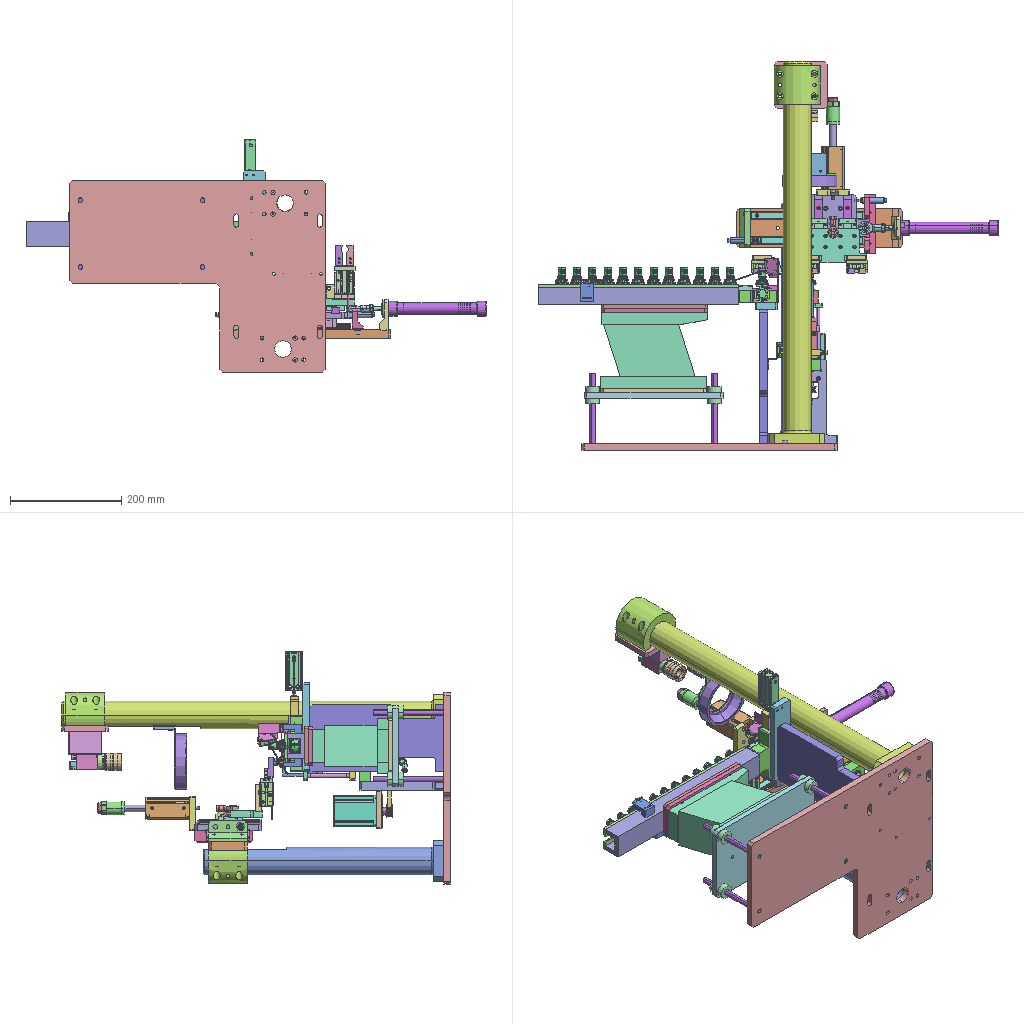Assembly | STEP file | 91 different items | 145 placed | box 828 x 700 x 418 mm
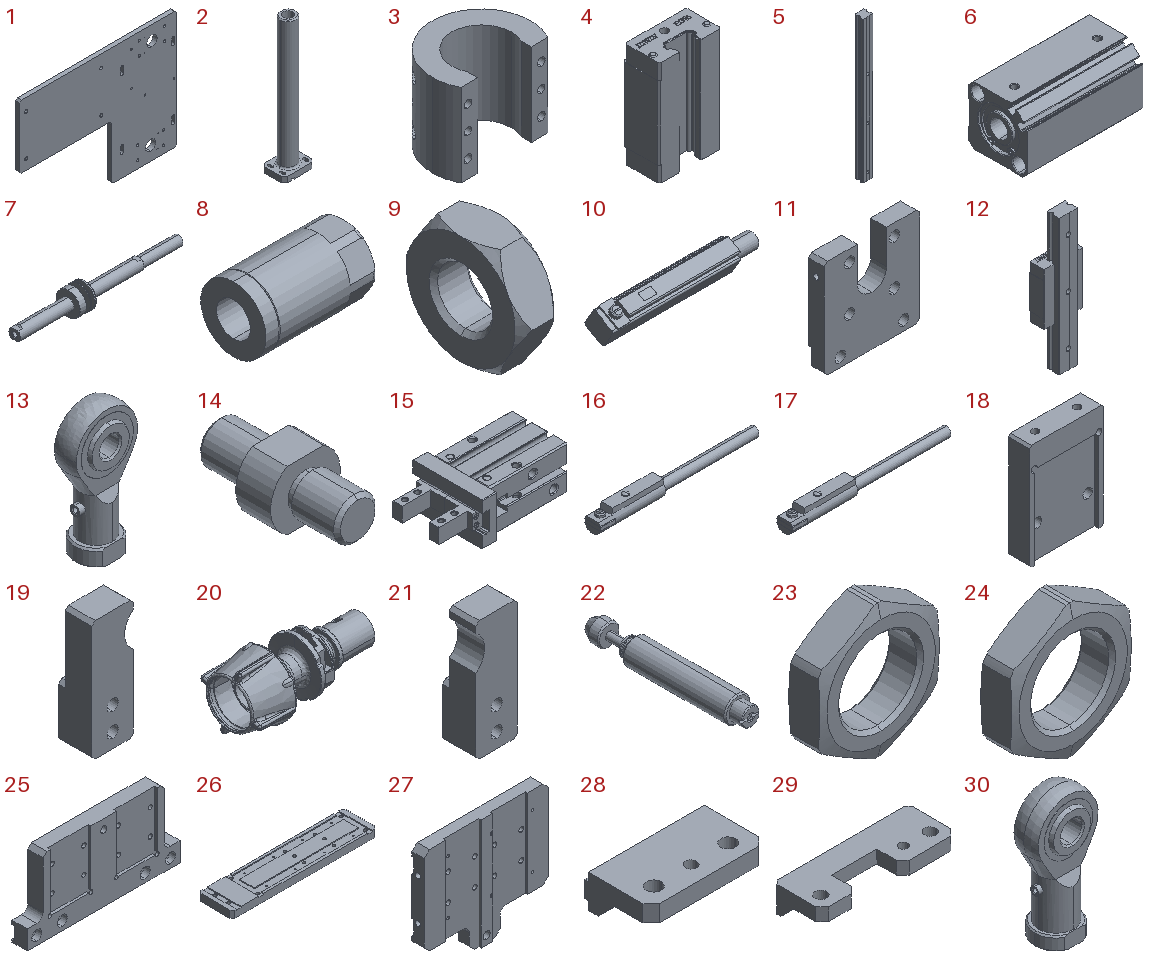Parts list (item | name | quantity | parent item | size | volume):
1 | PN_0009 | x1 | - | 460 x 12 x 345 mm | 1349018 mm3
2 | PN_0012 | x1 | in PN_0011 | 100 x 75 x 433 mm | 612416 mm3
3 | PN_0003 | x2 | in PN_0011, PN_0020 | 83 x 61 x 70 mm | 151269 mm3
4 | EGH15CA_BLOCK | x2 | in EGH15CA-220-2 | 34 x 19.5 x 57.8 mm | 30496 mm3
5 | EG15_RAIL-200 | x2 | in EGH15CA-220-2 | 15 x 12.5 x 200 mm | 32053 mm3
6 | ACQJS-25x40-20-G-11 | x1 | in ACQJS-25x40-20-G-1 (00) | 79 x 40 x 40 mm | 79327 mm3
7 | ACQJS-25x40-20-G-12 | x1 | in ACQJS-25x40-20-G-1 (00) | 170.5 x 25 x 25 mm | 21717 mm3
8 | ACQJS-25x40-20-G-13 | x1 | in ACQJS-25x40-20-G-1 (00) | 41 x 24 x 24 mm | 13745 mm3
9 | ACQJS-25x40-20-G-14 | x1 | in ACQJS-25x40-20-G-1 (00) | 6 x 19.63 x 17 mm | 1118 mm3
10 | ACQJS-25x40-20-G-15 | x1 | in ACQJS-25x40-20-G-1 (00) | 30.5 x 5.877 x 6.057 mm | 552.742 mm3
11 | PN_0013 | x1 | in PN_0011 | 60 x 10 x 62 mm | 28419 mm3
12 | MGN15C | x2 | in PN_0011 | 32 x 16 x 110 mm | 27183 mm3
13 | F-M06100U1 | x1 | in PN_0011 | - | 3624 mm3
14 | PN_0004 | x1 | in PN_0011 | 10 x 20 x 8.5 mm | 768.323 mm3
15 | HFZ16-B--BCL-H-21 | x3 | in HFZ16-B--BCL-H-2 | 67.3 x 38 x 23.6 mm | 30878 mm3
16 | HFZ16-B--BCL-H-22 | x3 | in HFZ16-B--BCL-H-2 | 42 x 4 x 5.1 mm | 360.74 mm3
17 | HFZ16-B--BCL-H-23 | x3 | in HFZ16-B--BCL-H-2 | 42 x 4 x 5.1 mm | 360.74 mm3
18 | PN_0014 | x3 | in PN_0011 | 35 x 10 x 50 mm | 14292 mm3
19 | PN_0015 | x3 | in PN_0011 | 12.5 x 10 x 36 mm | 3520 mm3
20 | Product 1 | x16 | in PN_0011, PN_0026, PN_0034, PN_0047 | 57.85 x 26.867 x 26.867 mm | 9145 mm3
21 | PN_0016 | x3 | in PN_0011 | 12.5 x 10 x 36 mm | 3520 mm3
22 | ACA-1007-11 | x2 | in ACA-1007-1 | 10 x 62 x 10 mm | 3798 mm3
23 | ACA-1007-12 | x2 | in ACA-1007-1 | 14 x 4 x 15.686 mm | 394.069 mm3
24 | ACA-1007-13 | x2 | in ACA-1007-1 | 14 x 4 x 15.686 mm | 394.069 mm3
25 | PN_0017 | x1 | in PN_0011 | 120 x 12 x 60 mm | 62781 mm3
26 | PN_0018 | x1 | in PN_0011 | 300 x 70 x 15 mm | 290778 mm3
27 | PN_0019 | x1 | in PN_0011 | 120 x 12 x 107.5 mm | 106389 mm3
28 | PN_0005 | x1 | in PN_0011 | 70 x 40 x 20 mm | 33206 mm3
29 | PN_0007 | x1 | in PN_0011 | 105 x 40 x 20 mm | 43466 mm3
30 | F-M08125U | x1 | in PN_0011 | 24 x 14 x 48 mm | 6722 mm3
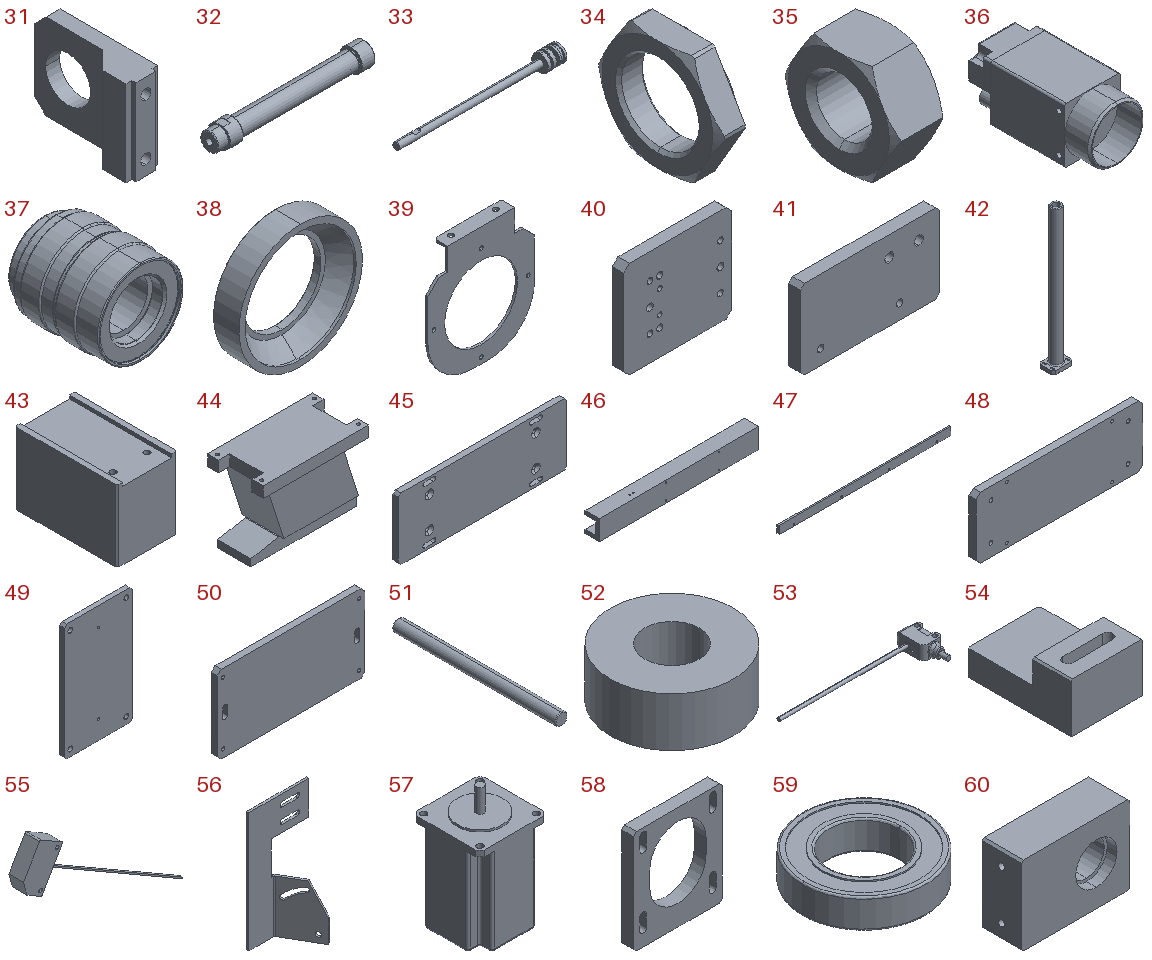31 | PN_0006 | x1 | in PN_0011 | 16 x 57 x 43 mm | 19963 mm3
32 | MA20x100-S-U1 | x1 | in MA20x100-S-U (0) | 188 x 27 x 27 mm | 33330 mm3
33 | MA20x100-S-U2 | x1 | in MA20x100-S-U (0) | 189 x 19.5 x 19.5 mm | 13401 mm3
34 | MA20x100-S-U3 | x1 | in MA20x100-S-U (0) | 7 x 33 x 29 mm | 2695 mm3
35 | MA20x100-S-U4 | x1 | in MA20x100-S-U (0) | 6 x 13.856 x 12 mm | 526.038 mm3
36 | MVC1000MF-M00 camera | x1 | in PN_0020 | 29 x 63.7 x 29 mm | 38507 mm3
37 | LTABA30_LTABA30 | x1 | in PN_0020 | 31 x 34 x 31 mm | 15140 mm3
38 | WLDR-LA100-W light source | x1 | in PN_0020 | 100 x 21 x 100 mm | 62526 mm3
39 | PN_0021 | x1 | in PN_0020 | 95 x 12 x 106 mm | 11586 mm3
40 | PN_0022 | x1 | in PN_0020 | 95 x 10 x 85 mm | 77581 mm3
41 | PN_0023 | x1 | in PN_0020 | 70 x 6 x 40 mm | 16459 mm3
42 | PN_0024 | x1 | in PN_0020 | 100 x 75 x 688 mm | 922519 mm3
43 | PN_0025 | x1 | in PN_0020 | 35 x 60 x 42 mm | 82188 mm3
44 | - | x1 | in PN_0026 | 192 x 100 x 136 mm | 1518745 mm3
45 | PN_0027 | x1 | in PN_0026 | 190 x 6 x 70 mm | 77614 mm3
46 | PN_0028 | x1 | in PN_0026 | 360 x 31.8 x 45 mm | 274443 mm3
47 | PN_0029 | x2 | in PN_0026 | 360 x 5.4 x 16.8 mm | 31743 mm3
48 | PN_0030 | x1 | in PN_0026 | 190 x 8 x 70 mm | 104613 mm3
49 | PN_0031 | x1 | in PN_0026 | 145 x 10 x 250 mm | 358144 mm3
50 | PN_0032 | x1 | in PN_0026 | 190 x 8 x 100 mm | 149586 mm3
51 | PN_0002 | x4 | in PN_0026 | 10 x 135 x 10 mm | 10595 mm3
52 | PN_0008 | x8 | in PN_0026 | 25 x 25 x 10 mm | 3958 mm3
53 | E3T-ST11 | x2 | in PN_0026 | 74.901 x 22.575 x 7 mm | 1025 mm3
54 | PN_0033 | x2 | in PN_0026 | 22.5 x 32.5 x 15.5 mm | 7082 mm3
55 | optexzd-l40n | x1 | - | 125.041 x 11 x 83.373 mm | 6875 mm3
56 | PN_0010 | x1 | - | 40 x 24.566 x 80 mm | 3826 mm3
57 | 57HS13_1 | x1 | in PN_0034 | 56.5 x 56.5 x 99 mm | 221285 mm3
58 | PN_0035 | x1 | in PN_0034 | 60 x 8 x 70 mm | 19436 mm3
59 | C-B6801ZZ_1 | x2 | in PN_0034 | 21 x 21 x 5 mm | 1103 mm3
60 | PN_0036 | x1 | in PN_0034 | 55 x 20 x 40 mm | 37681 mm3
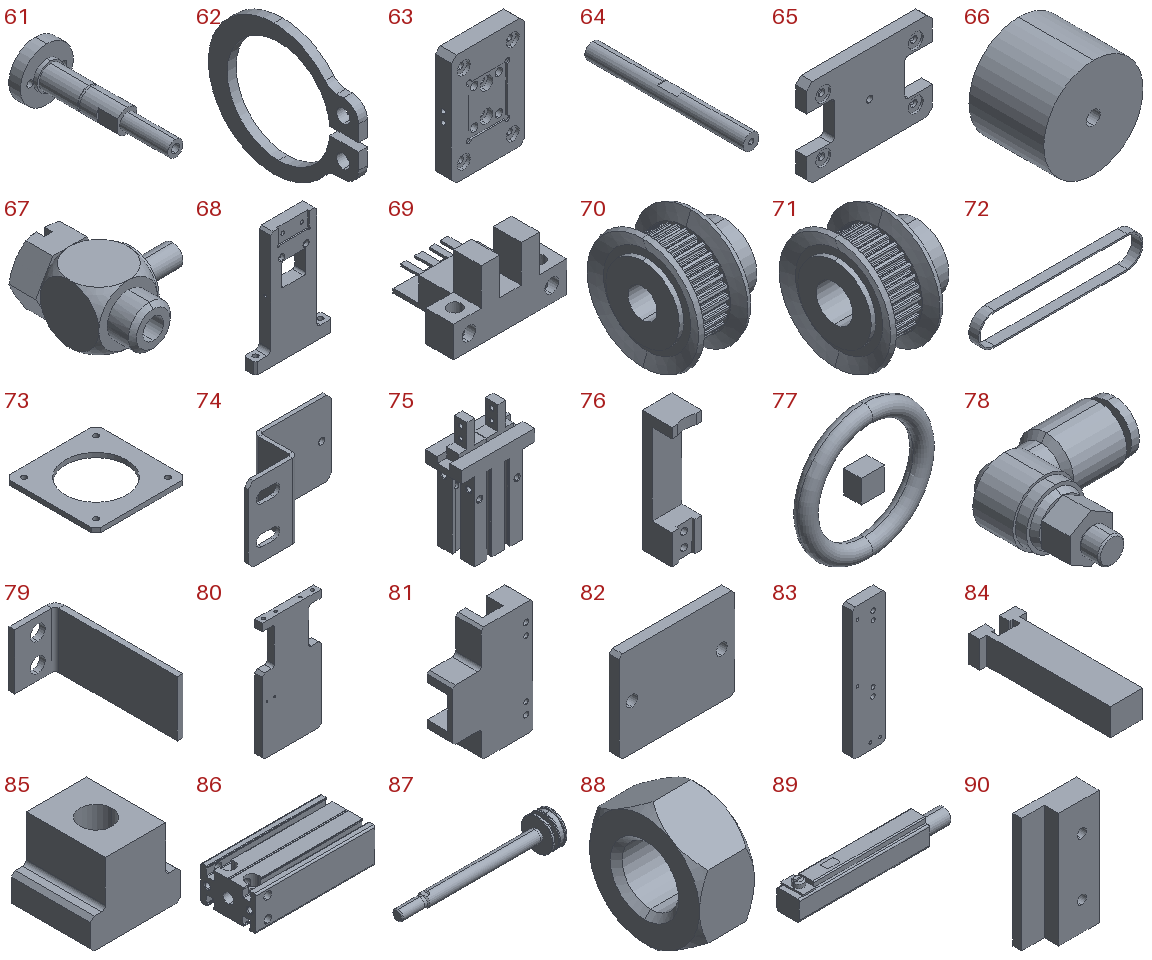61 | PN_0037 | x1 | in PN_0034 | 27.5 x 73 x 27.5 mm | 9090 mm3
62 | STWN12_1 | x1 | in PN_0034 | 1 x 16.8 x 14.65 mm | 77.172 mm3
63 | PN_0038 | x1 | in PN_0034 | 45 x 10 x 68 mm | 26101 mm3
64 | PN_0039 | x4 | in PN_0034 | 8 x 80 x 8 mm | 3898 mm3
65 | PN_0040 | x1 | in PN_0034 | 68 x 6 x 47.5 mm | 14110 mm3
66 | PN_0041 | x1 | in PN_0034 | 32.5 x 24.5 x 32.5 mm | 9394 mm3
67 | MS-5ALHU-4 | x2 | in PN_0034 | - | -
68 | PN_0042 | x1 | in PN_0034 | 100 x 15 x 152 mm | 126808 mm3
69 | EE-SX-671 | x1 | in PN_0034 | 26.4 x 20.5 x 15.8 mm | 2357 mm3
70 | ATP30MXL025-B-P6.35 | x1 | in PN_0034 | 18 x 25 x 25 mm | 3723 mm3
71 | ATP30MXL025-B-P8 | x1 | in PN_0034 | 18 x 25 x 25 mm | 3402 mm3
72 | MXL-025-118 | x1 | in PN_0034 | 110.4 x 6.4 x 21.4 mm | 1549 mm3
73 | PN_0043 | x1 | in PN_0034 | 60 x 60 x 3 mm | 6873 mm3
74 | PN_0044 | x1 | in PN_0034 | 48.5 x 16.5 x 30 mm | 2658 mm3
75 | MHZL2-16S (14.9) | x1 | in PN_0034 | 47 x 23.6 x 75 mm | 38591 mm3
76 | PN_0045 | x2 | in PN_0034 | 15 x 15 x 61 mm | 6956 mm3
77 | O-ring ID 8.5 x 1.5 | x1 | in PN_0034 | 11.5 x 1.5 x 11.5 mm | 61.517 mm3
78 | KSL04-M5 | x1 | in PN_0034 | 27 x 25.7 x 12 mm | 2672 mm3
79 | PN_0046 | x1 | in PN_0034 | 10 x 27.5 x 12 mm | 495.157 mm3
80 | PN_0048 | x1 | in PN_0047 | 120 x 15 x 241.5 mm | 375920 mm3
81 | PN_0049 | x1 | in PN_0047 | 70 x 22.5 x 100 mm | 72311 mm3
82 | PN_0050 | x1 | in PN_0047 | 35 x 3 x 27.5 mm | 2827 mm3
83 | PN_0051 | x1 | in PN_0047 | 40 x 12 x 160 mm | 74451 mm3
84 | PN_0052 | x1 | in PN_0047 | 26 x 75 x 15 mm | 19589 mm3
85 | PN_0001 | x1 | in PN_0047 | 12 x 10.5 x 10 mm | 865.332 mm3
86 | MD-16x30-S-G-11 | x1 | in MD-16x30-S-G-1 (0) | 70 x 32.2 x 20.2 mm | 27511 mm3
87 | MD-16x30-S-G-12 | x1 | in MD-16x30-S-G-1 (0) | 77 x 15.6 x 15.6 mm | 3019 mm3
88 | MD-16x30-S-G-13 | x1 | in MD-16x30-S-G-1 (0) | 4 x 8 x 9.238 mm | 163.482 mm3
89 | MD-16x30-S-G-14 | x1 | in MD-16x30-S-G-1 (0) | 30.5 x 4.4 x 5.5 mm | 552.742 mm3
90 | PN_0053 | x1 | in PN_0047 | 22 x 8 x 40 mm | 5311 mm3
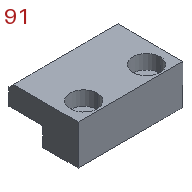91 | PN_0054 | x2 | in PN_0047 | 25 x 16.5 x 9.5 mm | 2670 mm3
Placements (level | parent | child | x y z in mm | rotation matrix by rows):
1 | subassembly 2 | PN_0009 | 16.37 -11.138 350.0 | 1 0 0 0 1 0 0 0 1
1 | subassembly 2 | PN_0011 | 167.298 -203.138 211.063 | -1 0 0 0 0 1 0 1 -0
2 | PN_0011 | PN_0012 | -2.882 7.937 213.0 | 1 0 0 0 1 0 0 0 1
2 | PN_0011 | PN_0003 | -2.882 7.937 592.5 | -1 0 0 0 -1 0 0 0 1
2 | PN_0011 | EGH15CA-220-2 | 43.163 122.169 601.791 | 0 0 -1 0 1 0 1 0 -0
3 | EGH15CA-220-2 | EGH15CA_BLOCK | 13.209 -57.762 94.745 | 1 0 0 0 1 0 0 0 1
3 | EGH15CA-220-2 | EG15_RAIL-200 | 13.209 -57.732 18.045 | 1 0 0 0 1 0 0 0 1
2 | PN_0011 | ACQJS-25x40-20-G-1 (00) | -71.482 102.907 661.0 | 0 0 1 0 -1 0 1 0 0
3 | ACQJS-25x40-20-G-1 (00) | ACQJS-25x40-20-G-11 | 0.0 0.0 0.0 | 1 0 0 0 1 0 0 0 1
3 | ACQJS-25x40-20-G-1 (00) | ACQJS-25x40-20-G-12 | 0.0 0.0 0.0 | 1 0 0 0 1 0 0 0 1
3 | ACQJS-25x40-20-G-1 (00) | ACQJS-25x40-20-G-13 | 0.0 0.0 0.0 | 1 0 0 0 1 0 0 0 1
3 | ACQJS-25x40-20-G-1 (00) | ACQJS-25x40-20-G-14 | 0.0 0.0 0.0 | 1 0 0 0 1 0 0 0 1
3 | ACQJS-25x40-20-G-1 (00) | ACQJS-25x40-20-G-15 | 0.0 0.0 0.0 | 1 0 0 0 1 0 0 0 1
2 | PN_0011 | PN_0013 | -71.482 93.407 661.0 | 1 0 0 0 0 1 0 -1 0
2 | PN_0011 | MGN15C | -45.482 72.407 588.0 | 1 0 0 0 1 0 0 0 1
2 | PN_0011 | F-M06100U1 | -71.482 102.907 613.5 | -1 0 0 0 1 0 0 0 -1
2 | PN_0011 | PN_0004 | -71.482 102.907 656.0 | 0.9804 0 0.1969 -0.1969 0 0.9804 0 -1 0
2 | PN_0011 | HFZ16-B--BCL-H-2 | -28.982 106.907 523.2 | 0 -1 0 -1 0 0 0 0 -1
3 | HFZ16-B--BCL-H-2 | HFZ16-B--BCL-H-21 | -0.0 0.0 -0.0 | 1 0 0 0 1 0 0 0 1
3 | HFZ16-B--BCL-H-2 | HFZ16-B--BCL-H-22 | -0.0 0.0 -0.0 | 1 0 0 0 1 0 0 0 1
3 | HFZ16-B--BCL-H-2 | HFZ16-B--BCL-H-23 | -0.0 0.0 -0.0 | 1 0 0 0 1 0 0 0 1
2 | PN_0011 | PN_0014 | -28.982 121.407 533.0 | 1 0 0 0 0 -1 0 1 -0
2 | PN_0011 | PN_0015 | -19.022 176.707 511.2 | -1 0 0 0 0 1 0 1 -0
2 | PN_0011 | Product 1 | -29.072 186.707 461.35 | 0 0.1559 0.9878 0 -0.9878 0.1559 1 0 0
2 | PN_0011 | PN_0016 | -38.942 176.707 511.2 | -1 0 0 0 0 1 0 1 -0
2 | PN_0011 | ACA-1007-1 | 118.618 69.437 570.0 | 0 -1 0 0.3818 0 0.9242 -0.9242 0 0.3818
3 | ACA-1007-1 | ACA-1007-11 | -0.0 -0.0 0.0 | 1 0 0 0 1 0 0 0 1
3 | ACA-1007-1 | ACA-1007-12 | -0.0 -0.0 0.0 | 1 0 0 0 1 0 0 0 1
3 | ACA-1007-1 | ACA-1007-13 | -0.0 -0.0 0.0 | 1 0 0 0 1 0 0 0 1
2 | PN_0011 | ACA-1007-1 | -168.382 69.437 642.5 | 0 1 0 -1 0 0 0 0 1
3 | ACA-1007-1 | ACA-1007-11 | -0.0 -0.0 0.0 | 1 0 0 0 1 0 0 0 1
3 | ACA-1007-1 | ACA-1007-12 | -0.0 -0.0 0.0 | 1 0 0 0 1 0 0 0 1
3 | ACA-1007-1 | ACA-1007-13 | -0.0 -0.0 0.0 | 1 0 0 0 1 0 0 0 1
2 | PN_0011 | PN_0016 | 46.058 176.707 511.2 | -1 0 0 0 0 1 0 1 -0
2 | PN_0011 | PN_0015 | 65.978 176.707 511.2 | -1 0 0 0 0 1 0 1 -0
2 | PN_0011 | PN_0017 | -71.482 86.407 561.0 | 1 0 0 0 1 0 0 0 1
2 | PN_0011 | MGN15C | -97.482 72.407 588.0 | 1 0 0 0 1 0 0 0 1
2 | PN_0011 | PN_0015 | -104.022 176.707 511.2 | -1 0 0 0 0 1 0 1 -0
2 | PN_0011 | PN_0016 | -123.942 176.707 511.2 | -1 0 0 0 0 1 0 1 -0
2 | PN_0011 | HFZ16-B--BCL-H-2 | -113.982 106.907 523.2 | 0 -1 0 -1 0 0 0 0 -1
3 | HFZ16-B--BCL-H-2 | HFZ16-B--BCL-H-21 | -0.0 0.0 -0.0 | 1 0 0 0 1 0 0 0 1
3 | HFZ16-B--BCL-H-2 | HFZ16-B--BCL-H-22 | -0.0 0.0 -0.0 | 1 0 0 0 1 0 0 0 1
3 | HFZ16-B--BCL-H-2 | HFZ16-B--BCL-H-23 | -0.0 0.0 -0.0 | 1 0 0 0 1 0 0 0 1
2 | PN_0011 | PN_0014 | -113.982 121.407 533.0 | 1 0 0 0 0 -1 0 1 -0
2 | PN_0011 | PN_0018 | -197.382 27.437 627.5 | 1 0 0 0 0 1 0 -1 0
2 | PN_0011 | EGH15CA-220-2 | 43.163 122.169 556.791 | 0 0 -1 0 1 0 1 0 -0
3 | EGH15CA-220-2 | EGH15CA_BLOCK | 13.209 -57.762 94.745 | 1 0 0 0 1 0 0 0 1
3 | EGH15CA-220-2 | EG15_RAIL-200 | 13.209 -57.732 18.045 | 1 0 0 0 1 0 0 0 1
2 | PN_0011 | PN_0019 | -28.982 62.407 653.0 | 0 0 1 0 1 0 -1 0 0
2 | PN_0011 | PN_0005 | 97.618 80.437 627.5 | 0 0 -1 0 -1 0 -1 0 -0
2 | PN_0011 | PN_0007 | -147.382 80.437 547.5 | 0 0 1 0 -1 0 1 0 0
2 | PN_0011 | F-M08125U | -164.482 80.407 592.5 | 0 0 1 0 -1 0 1 0 0
2 | PN_0011 | PN_0006 | -176.382 40.437 614.0 | -1 0 0 0 1 0 0 0 -1
2 | PN_0011 | MA20x100-S-U (0) | -208.382 80.437 592.5 | -1 0 0 0 -0.3818 0.9242 0 0.9242 0.3818
3 | MA20x100-S-U (0) | MA20x100-S-U1 | 0.0 0.0 0.0 | 1 0 0 0 1 0 0 0 1
3 | MA20x100-S-U (0) | MA20x100-S-U2 | 0.0 0.0 0.0 | 1 0 0 0 1 0 0 0 1
3 | MA20x100-S-U (0) | MA20x100-S-U3 | 0.0 0.0 0.0 | 1 0 0 0 1 0 0 0 1
3 | MA20x100-S-U (0) | MA20x100-S-U4 | 0.0 0.0 0.0 | 1 0 0 0 1 0 0 0 1
2 | PN_0011 | HFZ16-B--BCL-H-2 | 56.018 106.907 523.2 | 0 -1 0 -1 0 0 0 0 -1
3 | HFZ16-B--BCL-H-2 | HFZ16-B--BCL-H-21 | -0.0 0.0 -0.0 | 1 0 0 0 1 0 0 0 1
3 | HFZ16-B--BCL-H-2 | HFZ16-B--BCL-H-22 | -0.0 0.0 -0.0 | 1 0 0 0 1 0 0 0 1
3 | HFZ16-B--BCL-H-2 | HFZ16-B--BCL-H-23 | -0.0 0.0 -0.0 | 1 0 0 0 1 0 0 0 1
2 | PN_0011 | PN_0014 | 56.018 121.407 533.0 | 1 0 0 0 0 -1 0 1 -0
1 | subassembly 2 | PN_0020 | 83.167 197.583 504.878 | 0 0 1 0 1 0 -1 0 0
2 | PN_0020 | MVC1000MF-M00 camera | 107.108 425.78 113.203 | 0 0 1 0 1 0 -1 0 0
2 | PN_0020 | LTABA30_LTABA30 | 107.108 382.78 113.203 | 0 0 -1 0 1 0 1 0 0
2 | PN_0020 | WLDR-LA100-W light source | 107.108 265.78 113.203 | 0 0 -1 0 1 0 1 0 0
2 | PN_0020 | PN_0021 | 101.608 286.78 113.203 | 0 0 -1 0 1 0 1 0 0
2 | PN_0020 | PN_0022 | 52.608 448.78 97.5 | 0 -1 0 0 0 1 -1 0 0
2 | PN_0020 | PN_0023 | 48.608 306.28 108.203 | 0 -1 0 0 0 1 -1 0 0
2 | PN_0020 | PN_0024 | 23.108 -187.72 91.0 | 0 1 0 0 0 1 1 0 0
2 | PN_0020 | PN_0003 | 23.108 448.78 91.0 | 0 -1 0 0 0 1 -1 0 0
2 | PN_0020 | PN_0025 | 52.608 448.78 113.203 | 0 0 1 0 1 0 -1 0 0
1 | subassembly 2 | PN_0026 | -72.878 360.962 432.983 | -1 0 0 0 0 -1 0 -1 -0
2 | PN_0026 | subassembly 3 | 11.432 6.713 240.0 | 1 0 0 0 1 0 0 0 1
2 | PN_0026 | PN_0027 | 9.432 6.713 116.0 | 1 0 0 0 0 1 0 -1 0
2 | PN_0026 | PN_0028 | 39.432 6.713 110.0 | -1 0 0 0 0 -1 0 -1 -0
2 | PN_0026 | Product 1 | -126.768 6.713 101.58 | 0 -0.08761 0.9962 0 0.9962 0.08761 -1 0 0
2 | PN_0026 | PN_0029 | 39.432 -7.388 78.2 | 1 0 0 0 0 1 0 -1 0
2 | PN_0026 | Product 1 | -99.168 6.713 101.58 | 0 -0.08761 0.9962 0 0.9962 0.08761 -1 0 0
2 | PN_0026 | Product 1 | -71.568 6.713 101.58 | 0 -0.08761 0.9962 0 0.9962 0.08761 -1 0 0
2 | PN_0026 | Product 1 | -43.968 6.713 101.58 | 0 -0.08761 0.9962 0 0.9962 0.08761 -1 0 0
2 | PN_0026 | Product 1 | -16.368 6.713 101.58 | 0 -0.08761 0.9962 0 0.9962 0.08761 -1 0 0
2 | PN_0026 | Product 1 | 11.232 6.713 101.58 | 0 -0.08761 0.9962 0 0.9962 0.08761 -1 0 0
2 | PN_0026 | Product 1 | 38.832 6.713 101.58 | 0 -0.08761 0.9962 0 0.9962 0.08761 -1 0 0
2 | PN_0026 | Product 1 | 66.432 6.713 101.58 | 0 -0.08761 0.9962 0 0.9962 0.08761 -1 0 0
2 | PN_0026 | Product 1 | 94.032 6.713 101.58 | 0 -0.08761 0.9962 0 0.9962 0.08761 -1 0 0
2 | PN_0026 | Product 1 | 121.632 6.713 101.58 | 0 -0.08761 0.9962 0 0.9962 0.08761 -1 0 0
2 | PN_0026 | Product 1 | 149.232 6.713 101.58 | 0 -0.08761 0.9962 0 0.9962 0.08761 -1 0 0
2 | PN_0026 | Product 1 | 176.832 6.713 101.58 | 0 -0.08761 0.9962 0 0.9962 0.08761 -1 0 0
2 | PN_0026 | PN_0030 | 9.432 6.713 124.0 | 1 0 0 0 0 1 0 -1 0
2 | PN_0026 | PN_0031 | 11.432 6.713 278.0 | 0 0 -1 1 0 0 0 -1 -0
2 | PN_0026 | PN_0032 | 11.432 6.713 260.0 | 1 0 0 0 0 -1 0 1 -0
2 | PN_0026 | PN_0002 | 121.432 -53.288 368.054 | 0.8541 0 -0.5202 0.5202 0 0.8541 0 -1 0
2 | PN_0026 | PN_0008 | 121.432 -53.288 278.0 | 1 0 0 0 1 0 0 0 1
2 | PN_0026 | PN_0008 | 121.432 -53.288 258.0 | 1 0 0 0 1 0 0 0 1
2 | PN_0026 | PN_0008 | 121.432 66.713 278.0 | 1 0 0 0 1 0 0 0 1
2 | PN_0026 | PN_0008 | -98.568 -53.288 278.0 | 1 0 0 0 1 0 0 0 1
2 | PN_0026 | PN_0008 | -98.568 66.713 278.0 | 1 0 0 0 1 0 0 0 1
2 | PN_0026 | PN_0002 | 121.432 66.713 368.054 | 0.8541 0 -0.5202 0.5202 0 0.8541 0 -1 0
2 | PN_0026 | PN_0002 | -98.568 -53.288 368.054 | 0.8541 0 -0.5202 0.5202 0 0.8541 0 -1 0
2 | PN_0026 | PN_0002 | -98.568 66.713 368.054 | 0.8541 0 -0.5202 0.5202 0 0.8541 0 -1 0
2 | PN_0026 | PN_0008 | 121.432 66.713 258.0 | 1 0 0 0 1 0 0 0 1
2 | PN_0026 | PN_0008 | -98.568 -53.288 258.0 | 1 0 0 0 1 0 0 0 1
2 | PN_0026 | PN_0008 | -98.568 66.713 258.0 | 1 0 0 0 1 0 0 0 1
2 | PN_0026 | PN_0029 | 39.432 20.812 78.2 | -1 0 0 0 0 -1 0 -1 -0
2 | PN_0026 | E3T-ST11 | -53.363 -56.632 64.5 | 0.4226 0.9063 0 -0.9063 0.4226 0 0 0 1
2 | PN_0026 | E3T-ST11 | 288.746 70.057 64.5 | -0.4226 -0.9063 0 0.9063 -0.4226 0 0 0 1
2 | PN_0026 | PN_0033 | 103.823 44.712 87.75 | -1 0 0 0 0 -1 0 -1 -0
2 | PN_0026 | PN_0033 | 131.56 -31.288 87.75 | 1 0 0 0 0 1 0 -1 0
1 | subassembly 2 | optexzd-l40n | 524.355 1525.202 1848.934 | -0.5935 0.5 0.6307 -0.7282 0 -0.6853 -0.3427 -0.866 0.3641
1 | subassembly 2 | PN_0010 | 138.69 294.462 458.142 | 0 1 0 0 0 -1 -1 0 0
1 | subassembly 2 | PN_0034 | 191.5 -42.542 403.297 | 1 0 0 0 0 1 0 -1 0
2 | PN_0034 | 57HS13_1 | 4.871 94.527 164.404 | 1 0 0 0 -1 0 0 0 -1
2 | PN_0034 | PN_0035 | 4.871 91.527 164.404 | 1 0 0 0 0 1 0 -1 0
2 | PN_0034 | C-B6801ZZ_1 | 4.871 5.527 175.404 | -0.9237 -0.383 0 -0.383 0.9237 0 0 0 -1
2 | PN_0034 | C-B6801ZZ_1 | 4.871 5.527 190.404 | 0.9237 0.383 0 0.383 -0.9237 0 0 0 -1
2 | PN_0034 | PN_0036 | 4.871 16.027 175.404 | 0 0 -1 -1 0 0 0 1 0
2 | PN_0034 | PN_0037 | 4.871 5.527 130.404 | 0 0 -1 -1 0 0 0 1 0
2 | PN_0034 | STWN12_1 | 4.871 5.002 174.754 | 0 0 1 0 1 0 -1 0 0
2 | PN_0034 | PN_0038 | 4.871 5.527 212.404 | 1 0 0 0 0 1 0 -1 0
2 | PN_0034 | PN_0039 | -10.129 30.527 250.404 | 1 0 0 0 0 -1 0 1 0
2 | PN_0034 | PN_0039 | 19.871 30.527 250.404 | 1 0 0 0 0 -1 0 1 0
2 | PN_0034 | PN_0039 | -10.129 -19.473 250.404 | 1 0 0 0 0 -1 0 1 0
2 | PN_0034 | PN_0039 | 19.871 -19.473 250.404 | 1 0 0 0 0 -1 0 1 0
2 | PN_0034 | PN_0040 | 4.871 5.527 289.404 | 0 0 -1 -1 0 0 0 1 -0
2 | PN_0034 | PN_0041 | 4.871 5.527 294.404 | -0.1825 0 0.9832 0.9832 0 0.1825 0 1 0
2 | PN_0034 | Product 1 | 4.871 5.527 300.724 | 0 0 1 0 -1 0 1 0 0
2 | PN_0034 | MS-5ALHU-4 | 27.371 5.527 207.404 | 0 1 0 -1 0 0 0 0 1
2 | PN_0034 | MS-5ALHU-4 | 11.371 -9.773 242.404 | -1 0 0 0 -1 0 0 0 1
2 | PN_0034 | PN_0042 | 4.871 41.527 126.904 | 1 0 0 0 1 0 0 0 1
2 | PN_0034 | EE-SX-671 | -420.329 75.777 119.604 | 0 0 1 0 -1 0 1 0 -0
2 | PN_0034 | ATP30MXL025-B-P6.35 | 4.871 94.527 135.404 | 0 -0.0184 -0.9998 0 0.9998 -0.0184 1 0 -0
2 | PN_0034 | ATP30MXL025-B-P8 | 4.871 5.527 135.404 | 0 0.334 0.9426 0 -0.9426 0.334 1 0 -0
2 | PN_0034 | MXL-025-118 | 4.871 51.711 137.954 | 0 0 -1 -1 0 0 0 1 0
2 | PN_0034 | PN_0043 | 4.871 94.527 153.404 | 1 0 0 0 1 0 0 0 1
2 | PN_0034 | PN_0044 | -53.329 -9.473 195.454 | 0 1 0 0 0 1 1 0 0
2 | PN_0034 | MHZL2-16S (14.9) | 4.871 5.527 270.104 | 0 1 0 -1 0 0 0 0 1
2 | PN_0034 | PN_0045 | 4.871 16.477 302.904 | 1 0 0 0 1 0 0 0 1
2 | PN_0034 | PN_0045 | 4.871 -5.423 302.904 | -1 0 0 0 -1 0 0 0 1
2 | PN_0034 | O-ring ID 8.5 x 1.5 | 4.683 5.362 202.954 | -0.06804 0 0.9977 -0.9977 0 -0.06804 0 -1 -0
2 | PN_0034 | KSL04-M5 | 4.871 5.527 134.404 | -0.5507 0 -0.8347 0.8347 0 -0.5507 0 -1 0
2 | PN_0034 | PN_0046 | -17.629 -0.4729 212.404 | 0 1 0 0 0 1 1 0 -0
1 | subassembly 2 | PN_0047 | 121.514 341.712 444.182 | 0 -1 0 0 0 -1 1 0 0
2 | PN_0047 | PN_0048 | -3.912 0.3237 220.0 | 1 0 0 0 1 0 0 0 1
2 | PN_0047 | PN_0049 | -13.912 5.324 87.25 | 0 0 1 -1 0 0 0 -1 0
2 | PN_0047 | PN_0050 | 22.338 10.324 64.75 | 0 0 1 -1 0 0 0 -1 0
2 | PN_0047 | PN_0051 | 16.088 2.824 99.25 | 0 0 -1 1 0 0 0 -1 -0
2 | PN_0047 | Product 1 | -46.412 10.324 83.53 | 0 -0.05375 0.9986 0 0.9986 0.05375 -1 0 0
2 | PN_0047 | PN_0052 | -3.412 10.324 72.25 | 0 1 0 -1 0 0 0 0 1
2 | PN_0047 | PN_0001 | 67.088 10.324 65.9 | 0 0 1 1 0 0 0 1 -0
2 | PN_0047 | MD-16x30-S-G-1 (0) | 81.088 10.324 71.15 | 1 0 0 0 0 -1 0 1 0
3 | MD-16x30-S-G-1 (0) | MD-16x30-S-G-11 | -0.0 -0.0 0.0 | 1 0 0 0 1 0 0 0 1
3 | MD-16x30-S-G-1 (0) | MD-16x30-S-G-12 | -0.0 -0.0 0.0 | 1 0 0 0 1 0 0 0 1
3 | MD-16x30-S-G-1 (0) | MD-16x30-S-G-13 | -0.0 -0.0 0.0 | 1 0 0 0 1 0 0 0 1
3 | MD-16x30-S-G-1 (0) | MD-16x30-S-G-14 | -0.0 -0.0 0.0 | 1 0 0 0 1 0 0 0 1
2 | PN_0047 | Product 1 | -17.912 10.324 83.53 | 0 -0.05375 0.9986 0 0.9986 0.05375 -1 0 0
2 | PN_0047 | PN_0053 | -11.678 -6.176 64.75 | 0 0 1 -1 0 0 0 -1 0
2 | PN_0047 | PN_0054 | -3.712 40.324 64.75 | 0 -1 0 -1 0 0 0 0 -1
2 | PN_0047 | PN_0054 | -32.112 40.324 64.75 | 0 1 0 1 0 0 0 0 -1